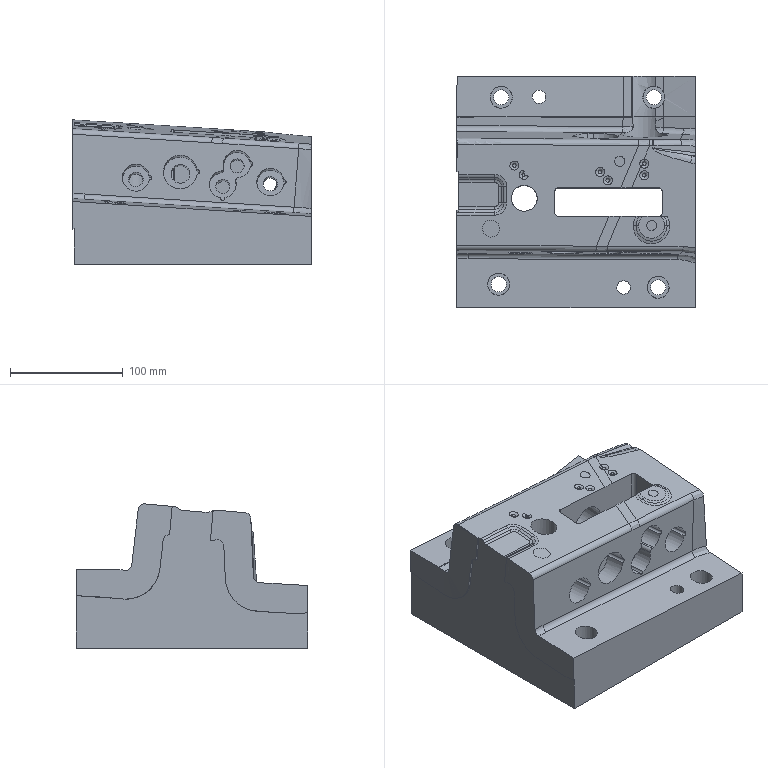Part | NX | features solid 2 | 1 solid | 186 faces | box 211.413 x 205 x 127.879 mm | volume 3233669 mm3 | cylinder 73 | spline 58 | plane 39 | torus 7 | sphere 6 | cone 3 | commonest cylinder face diameters 10 x15 24 x8 4 x7 40 x7 6 x6 13.5 x4